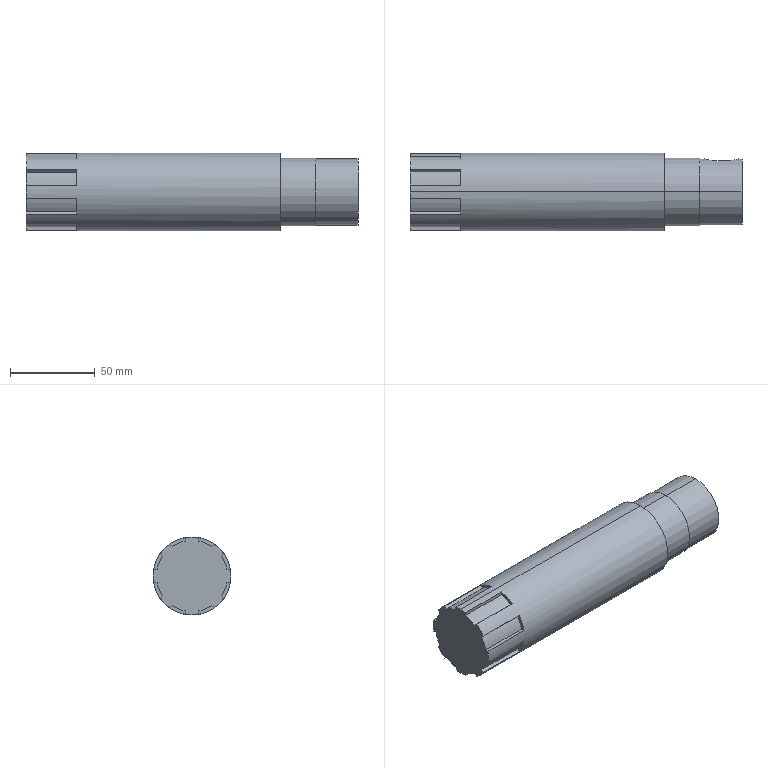Part | SolidWorks | features ICE 4, Extrusion 1, HoleWzd 1 | 1 solid | 51 faces | box 196 x 46 x 46 mm | volume 298815 mm3 | plane 31 | cylinder 18 | cone 2 | commonest cylinder face diameters 42.078 x8 8.5 x2 12 x2 39 x2 40 x2 46 x2